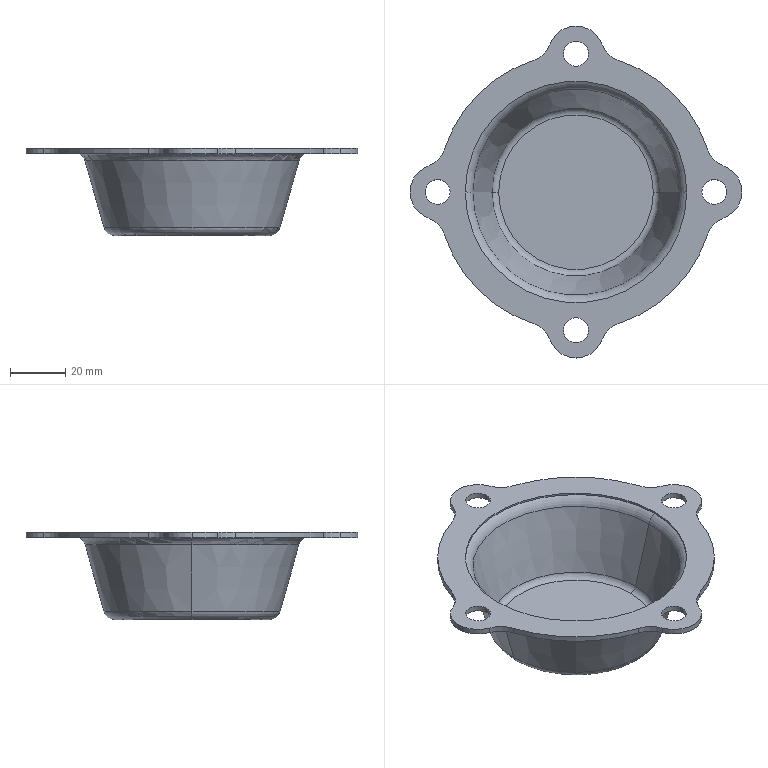Part | STEP file | AXIS_COVER1V11 | 1 solid | 43 faces | box 120 x 120 x 31.5 mm | volume 20879 mm3 | cylinder 27 | torus 8 | cone 4 | plane 4 | commonest cylinder face diameters 20 x13 9 x8 100 x4 80 x2